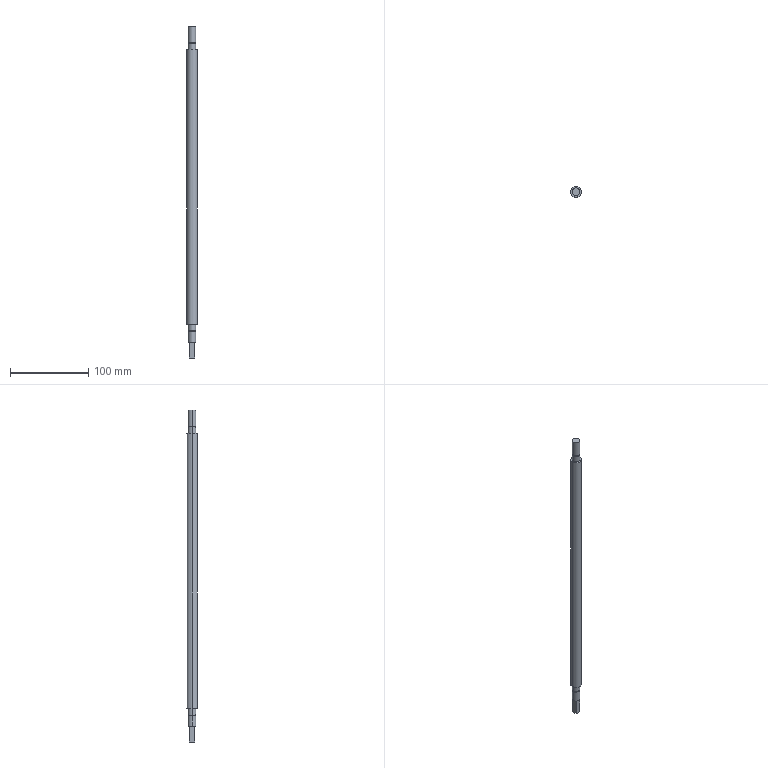Part | STEP file | 602-09-0048 | 1 solid | 27 faces | box 14 x 14 x 425 mm | volume 59315 mm3 | cylinder 14 | plane 13 | commonest cylinder face diameters 10 x8 9.6 x4 14 x2